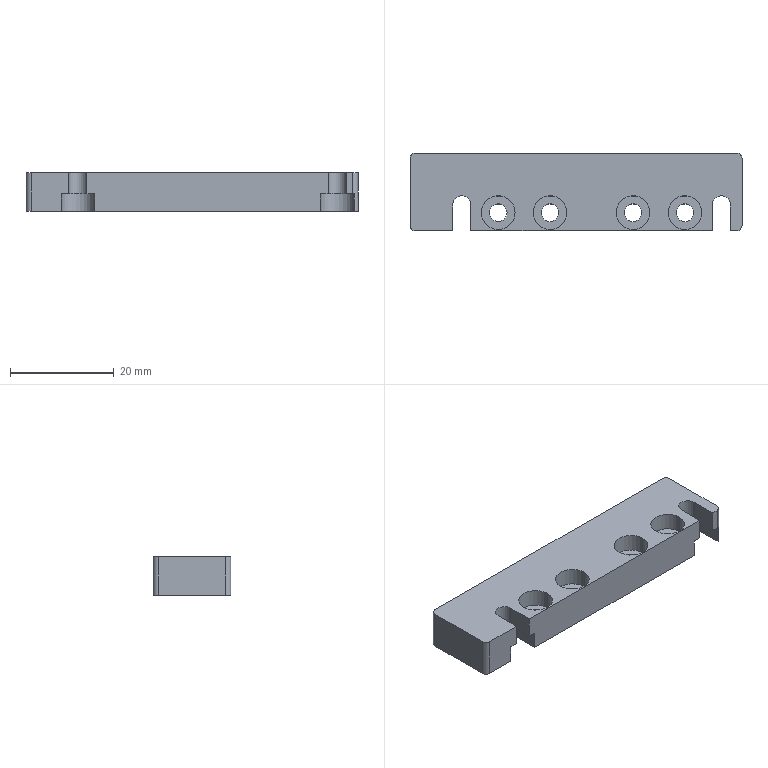Part | SolidWorks | features BaseBody 1 | 1 solid | 46 faces | box 64 x 15 x 7.5 mm | volume 6074 mm3 | cylinder 24 | plane 22 | commonest cylinder face diameters 6.5 x10 3.4 x8 2 x4 3.5 x2
STEP:
#1=CARTESIAN_POINT('',(-16.7,-4.,0.));
#2=VERTEX_POINT('',#1);
#3=CARTESIAN_POINT('',(-13.3,-4.,0.));
#4=VERTEX_POINT('',#3);
#5=CARTESIAN_POINT('',(-15.,-4.,0.));
#6=DIRECTION('',(0.,0.,1.));
#7=DIRECTION('',(1.,0.,0.));
#8=AXIS2_PLACEMENT_3D('',#5,#6,#7);
#9=CIRCLE('',#8,1.7);
#10=EDGE_CURVE('',#2,#4,#9,.T.);
#11=ORIENTED_EDGE('',*,*,#10,.F.);
#12=CARTESIAN_POINT('',(-16.7,-4.,4.1));
#13=VERTEX_POINT('',#12);
#14=CARTESIAN_POINT('',(-16.7,-4.,7.5));
#15=DIRECTION('',(0.,0.,1.));
#16=VECTOR('',#15,1000.);
#17=LINE('',#14,#16);
#18=EDGE_CURVE('',#2,#13,#17,.T.);
#19=ORIENTED_EDGE('',*,*,#18,.T.);
#20=CARTESIAN_POINT('',(-13.3,-4.,4.1));
#21=VERTEX_POINT('',#20);
#22=CARTESIAN_POINT('',(-15.,-4.,4.1));
#23=DIRECTION('',(0.,0.,-1.));
#24=DIRECTION('',(1.,0.,0.));
#25=AXIS2_PLACEMENT_3D('',#22,#23,#24);
#26=CIRCLE('',#25,1.7);
#27=EDGE_CURVE('',#21,#13,#26,.T.);
#28=ORIENTED_EDGE('',*,*,#27,.F.);
#29=CARTESIAN_POINT('',(-13.3,-4.,7.5));
#30=DIRECTION('',(0.,0.,1.));
#31=VECTOR('',#30,1000.);
#32=LINE('',#29,#31);
#33=EDGE_CURVE('',#4,#21,#32,.T.);
#34=ORIENTED_EDGE('',*,*,#33,.F.);
#35=EDGE_LOOP('',(#11,#19,#28,#34));
#36=FACE_OUTER_BOUND('',#35,.T.);
#37=CARTESIAN_POINT('',(-15.,-4.,7.5));
#38=DIRECTION('',(0.,0.,1.));
#39=DIRECTION('',(1.,0.,0.));
#40=AXIS2_PLACEMENT_3D('',#37,#38,#39);
#41=CYLINDRICAL_SURFACE('',#40,1.7);
#42=ADVANCED_FACE('',(#36),#41,.F.);
#43=CARTESIAN_POINT('',(9.3,-4.,0.));
#44=VERTEX_POINT('',#43);
#45=CARTESIAN_POINT('',(12.7,-4.,0.));
#46=VERTEX_POINT('',#45);
#47=CARTESIAN_POINT('',(11.,-4.,0.));
#48=DIRECTION('',(0.,0.,1.));
#49=DIRECTION('',(1.,0.,0.));
#50=AXIS2_PLACEMENT_3D('',#47,#48,#49);
#51=CIRCLE('',#50,1.7);
#52=EDGE_CURVE('',#44,#46,#51,.T.);
#53=ORIENTED_EDGE('',*,*,#52,.F.);
#54=CARTESIAN_POINT('',(9.3,-4.,4.1));
#55=VERTEX_POINT('',#54);
#56=CARTESIAN_POINT('',(9.3,-4.,7.5));
#57=DIRECTION('',(0.,0.,1.));
#58=VECTOR('',#57,1000.);
#59=LINE('',#56,#58);
#60=EDGE_CURVE('',#44,#55,#59,.T.);
#61=ORIENTED_EDGE('',*,*,#60,.T.);
#62=CARTESIAN_POINT('',(12.7,-4.,4.1));
#63=VERTEX_POINT('',#62);
#64=CARTESIAN_POINT('',(11.,-4.,4.1));
#65=DIRECTION('',(0.,0.,-1.));
#66=DIRECTION('',(1.,0.,0.));
#67=AXIS2_PLACEMENT_3D('',#64,#65,#66);
#68=CIRCLE('',#67,1.7);
#69=EDGE_CURVE('',#63,#55,#68,.T.);
#70=ORIENTED_EDGE('',*,*,#69,.F.);
#71=CARTESIAN_POINT('',(12.7,-4.,7.5));
#72=DIRECTION('',(0.,0.,1.));
#73=VECTOR('',#72,1000.);
#74=LINE('',#71,#73);
#75=EDGE_CURVE('',#46,#63,#74,.T.);
#76=ORIENTED_EDGE('',*,*,#75,.F.);
#77=EDGE_LOOP('',(#53,#61,#70,#76));
#78=FACE_OUTER_BOUND('',#77,.T.);
#79=CARTESIAN_POINT('',(11.,-4.,7.5));
#80=DIRECTION('',(0.,0.,1.));
#81=DIRECTION('',(1.,0.,0.));
#82=AXIS2_PLACEMENT_3D('',#79,#80,#81);
#83=CYLINDRICAL_SURFACE('',#82,1.7);
#84=ADVANCED_FACE('',(#78),#83,.F.);
#85=CARTESIAN_POINT('',(-6.7,-4.,0.));
#86=VERTEX_POINT('',#85);
#87=CARTESIAN_POINT('',(-3.3,-4.,0.));
#88=VERTEX_POINT('',#87);
#89=CARTESIAN_POINT('',(-5.,-4.,0.));
#90=DIRECTION('',(0.,0.,1.));
#91=DIRECTION('',(1.,0.,0.));
#92=AXIS2_PLACEMENT_3D('',#89,#90,#91);
#93=CIRCLE('',#92,1.7);
#94=EDGE_CURVE('',#86,#88,#93,.T.);
#95=ORIENTED_EDGE('',*,*,#94,.F.);
#96=CARTESIAN_POINT('',(-6.7,-4.,4.1));
#97=VERTEX_POINT('',#96);
#98=CARTESIAN_POINT('',(-6.7,-4.,7.5));
#99=DIRECTION('',(0.,0.,1.));
#100=VECTOR('',#99,1000.);
#101=LINE('',#98,#100);
#102=EDGE_CURVE('',#86,#97,#101,.T.);
#103=ORIENTED_EDGE('',*,*,#102,.T.);
#104=CARTESIAN_POINT('',(-3.3,-4.,4.1));
#105=VERTEX_POINT('',#104);
#106=CARTESIAN_POINT('',(-5.,-4.,4.1));
#107=DIRECTION('',(0.,0.,-1.));
#108=DIRECTION('',(1.,0.,0.));
#109=AXIS2_PLACEMENT_3D('',#106,#107,#108);
#110=CIRCLE('',#109,1.7);
#111=EDGE_CURVE('',#105,#97,#110,.T.);
#112=ORIENTED_EDGE('',*,*,#111,.F.);
#113=CARTESIAN_POINT('',(-3.3,-4.,7.5));
#114=DIRECTION('',(0.,0.,1.));
#115=VECTOR('',#114,1000.);
#116=LINE('',#113,#115);
#117=EDGE_CURVE('',#88,#105,#116,.T.);
#118=ORIENTED_EDGE('',*,*,#117,.F.);
#119=EDGE_LOOP('',(#95,#103,#112,#118));
#120=FACE_OUTER_BOUND('',#119,.T.);
#121=CARTESIAN_POINT('',(-5.,-4.,7.5));
#122=DIRECTION('',(0.,0.,1.));
#123=DIRECTION('',(1.,0.,0.));
#124=AXIS2_PLACEMENT_3D('',#121,#122,#123);
#125=CYLINDRICAL_SURFACE('',#124,1.7);
#126=ADVANCED_FACE('',(#120),#125,.F.);
#127=CARTESIAN_POINT('',(19.3,-4.,0.));
#128=VERTEX_POINT('',#127);
#129=CARTESIAN_POINT('',(22.7,-4.,0.));
#130=VERTEX_POINT('',#129);
#131=CARTESIAN_POINT('',(21.,-4.,0.));
#132=DIRECTION('',(0.,0.,1.));
#133=DIRECTION('',(1.,0.,0.));
#134=AXIS2_PLACEMENT_3D('',#131,#132,#133);
#135=CIRCLE('',#134,1.7);
#136=EDGE_CURVE('',#128,#130,#135,.T.);
#137=ORIENTED_EDGE('',*,*,#136,.F.);
#138=CARTESIAN_POINT('',(19.3,-4.,4.1));
#139=VERTEX_POINT('',#138);
#140=CARTESIAN_POINT('',(19.3,-4.,7.5));
#141=DIRECTION('',(0.,0.,1.));
#142=VECTOR('',#141,1000.);
#143=LINE('',#140,#142);
#144=EDGE_CURVE('',#128,#139,#143,.T.);
#145=ORIENTED_EDGE('',*,*,#144,.T.);
#146=CARTESIAN_POINT('',(22.7,-4.,4.1));
#147=VERTEX_POINT('',#146);
#148=CARTESIAN_POINT('',(21.,-4.,4.1));
#149=DIRECTION('',(0.,0.,-1.));
#150=DIRECTION('',(1.,0.,0.));
#151=AXIS2_PLACEMENT_3D('',#148,#149,#150);
#152=CIRCLE('',#151,1.7);
#153=EDGE_CURVE('',#147,#139,#152,.T.);
#154=ORIENTED_EDGE('',*,*,#153,.F.);
#155=CARTESIAN_POINT('',(22.7,-4.,7.5));
#156=DIRECTION('',(0.,0.,1.));
#157=VECTOR('',#156,1000.);
#158=LINE('',#155,#157);
#159=EDGE_CURVE('',#130,#147,#158,.T.);
#160=ORIENTED_EDGE('',*,*,#159,.F.);
#161=EDGE_LOOP('',(#137,#145,#154,#160));
#162=FACE_OUTER_BOUND('',#161,.T.);
#163=CARTESIAN_POINT('',(21.,-4.,7.5));
#164=DIRECTION('',(0.,0.,1.));
#165=DIRECTION('',(1.,0.,0.));
#166=AXIS2_PLACEMENT_3D('',#163,#164,#165);
#167=CYLINDRICAL_SURFACE('',#166,1.7);
#168=ADVANCED_FACE('',(#162),#167,.F.);
#169=CARTESIAN_POINT('',(-11.75,-4.,4.1));
#170=VERTEX_POINT('',#169);
#171=CARTESIAN_POINT('',(-18.25,-4.,4.1));
#172=VERTEX_POINT('',#171);
#173=CARTESIAN_POINT('',(-15.,-4.,4.1));
#174=DIRECTION('',(0.,0.,-1.));
#175=DIRECTION('',(1.,0.,0.));
#176=AXIS2_PLACEMENT_3D('',#173,#174,#175);
#177=CIRCLE('',#176,3.25);
#178=EDGE_CURVE('',#170,#172,#177,.T.);
#179=ORIENTED_EDGE('',*,*,#178,.T.);
#180=CARTESIAN_POINT('',(-18.25,-4.,7.5));
#181=VERTEX_POINT('',#180);
#182=CARTESIAN_POINT('',(-18.25,-4.,7.5));
#183=DIRECTION('',(0.,0.,1.));
#184=VECTOR('',#183,1000.);
#185=LINE('',#182,#184);
#186=EDGE_CURVE('',#172,#181,#185,.T.);
#187=ORIENTED_EDGE('',*,*,#186,.T.);
#188=CARTESIAN_POINT('',(-11.75,-4.,7.5));
#189=VERTEX_POINT('',#188);
#190=CARTESIAN_POINT('',(-15.,-4.,7.5));
#191=DIRECTION('',(0.,0.,1.));
#192=DIRECTION('',(1.,0.,0.));
#193=AXIS2_PLACEMENT_3D('',#190,#191,#192);
#194=CIRCLE('',#193,3.25);
#195=EDGE_CURVE('',#181,#189,#194,.T.);
#196=ORIENTED_EDGE('',*,*,#195,.T.);
#197=CARTESIAN_POINT('',(-11.75,-4.,7.5));
#198=DIRECTION('',(0.,0.,1.));
#199=VECTOR('',#198,1000.);
#200=LINE('',#197,#199);
#201=EDGE_CURVE('',#170,#189,#200,.T.);
#202=ORIENTED_EDGE('',*,*,#201,.F.);
#203=EDGE_LOOP('',(#179,#187,#196,#202));
#204=FACE_OUTER_BOUND('',#203,.T.);
#205=CARTESIAN_POINT('',(-15.,-4.,7.5));
#206=DIRECTION('',(0.,0.,1.));
#207=DIRECTION('',(1.,0.,0.));
#208=AXIS2_PLACEMENT_3D('',#205,#206,#207);
#209=CYLINDRICAL_SURFACE('',#208,3.25);
#210=ADVANCED_FACE('',(#204),#209,.F.);
#211=CARTESIAN_POINT('',(14.25,-4.,4.1));
#212=VERTEX_POINT('',#211);
#213=CARTESIAN_POINT('',(7.75,-4.,4.1));
#214=VERTEX_POINT('',#213);
#215=CARTESIAN_POINT('',(11.,-4.,4.1));
#216=DIRECTION('',(0.,0.,-1.));
#217=DIRECTION('',(1.,0.,0.));
#218=AXIS2_PLACEMENT_3D('',#215,#216,#217);
#219=CIRCLE('',#218,3.25);
#220=EDGE_CURVE('',#212,#214,#219,.T.);
#221=ORIENTED_EDGE('',*,*,#220,.T.);
#222=CARTESIAN_POINT('',(7.75,-4.,7.5));
#223=VERTEX_POINT('',#222);
#224=CARTESIAN_POINT('',(7.75,-4.,7.5));
#225=DIRECTION('',(0.,0.,1.));
#226=VECTOR('',#225,1000.);
#227=LINE('',#224,#226);
#228=EDGE_CURVE('',#214,#223,#227,.T.);
#229=ORIENTED_EDGE('',*,*,#228,.T.);
#230=CARTESIAN_POINT('',(14.25,-4.,7.5));
#231=VERTEX_POINT('',#230);
#232=CARTESIAN_POINT('',(11.,-4.,7.5));
#233=DIRECTION('',(0.,0.,1.));
#234=DIRECTION('',(1.,0.,0.));
#235=AXIS2_PLACEMENT_3D('',#232,#233,#234);
#236=CIRCLE('',#235,3.25);
#237=EDGE_CURVE('',#223,#231,#236,.T.);
#238=ORIENTED_EDGE('',*,*,#237,.T.);
#239=CARTESIAN_POINT('',(14.25,-4.,7.5));
#240=DIRECTION('',(0.,0.,1.));
#241=VECTOR('',#240,1000.);
#242=LINE('',#239,#241);
#243=EDGE_CURVE('',#212,#231,#242,.T.);
#244=ORIENTED_EDGE('',*,*,#243,.F.);
#245=EDGE_LOOP('',(#221,#229,#238,#244));
#246=FACE_OUTER_BOUND('',#245,.T.);
#247=CARTESIAN_POINT('',(11.,-4.,7.5));
#248=DIRECTION('',(0.,0.,1.));
#249=DIRECTION('',(1.,0.,0.));
#250=AXIS2_PLACEMENT_3D('',#247,#248,#249);
#251=CYLINDRICAL_SURFACE('',#250,3.25);
#252=ADVANCED_FACE('',(#246),#251,.F.);
#253=CARTESIAN_POINT('',(-1.75,-4.,4.1));
#254=VERTEX_POINT('',#253);
#255=CARTESIAN_POINT('',(-8.25,-4.,4.1));
#256=VERTEX_POINT('',#255);
#257=CARTESIAN_POINT('',(-5.,-4.,4.1));
#258=DIRECTION('',(0.,0.,-1.));
#259=DIRECTION('',(1.,0.,0.));
#260=AXIS2_PLACEMENT_3D('',#257,#258,#259);
#261=CIRCLE('',#260,3.25);
#262=EDGE_CURVE('',#254,#256,#261,.T.);
#263=ORIENTED_EDGE('',*,*,#262,.T.);
#264=CARTESIAN_POINT('',(-8.25,-4.,7.5));
#265=VERTEX_POINT('',#264);
#266=CARTESIAN_POINT('',(-8.25,-4.,7.5));
#267=DIRECTION('',(0.,0.,1.));
#268=VECTOR('',#267,1000.);
#269=LINE('',#266,#268);
#270=EDGE_CURVE('',#256,#265,#269,.T.);
#271=ORIENTED_EDGE('',*,*,#270,.T.);
#272=CARTESIAN_POINT('',(-1.75,-4.,7.5));
#273=VERTEX_POINT('',#272);
#274=CARTESIAN_POINT('',(-5.,-4.,7.5));
#275=DIRECTION('',(0.,0.,1.));
#276=DIRECTION('',(1.,0.,0.));
#277=AXIS2_PLACEMENT_3D('',#274,#275,#276);
#278=CIRCLE('',#277,3.25);
#279=EDGE_CURVE('',#265,#273,#278,.T.);
#280=ORIENTED_EDGE('',*,*,#279,.T.);
#281=CARTESIAN_POINT('',(-1.75,-4.,7.5));
#282=DIRECTION('',(0.,0.,1.));
#283=VECTOR('',#282,1000.);
#284=LINE('',#281,#283);
#285=EDGE_CURVE('',#254,#273,#284,.T.);
#286=ORIENTED_EDGE('',*,*,#285,.F.);
#287=EDGE_LOOP('',(#263,#271,#280,#286));
#288=FACE_OUTER_BOUND('',#287,.T.);
#289=CARTESIAN_POINT('',(-5.,-4.,7.5));
#290=DIRECTION('',(0.,0.,1.));
#291=DIRECTION('',(1.,0.,0.));
#292=AXIS2_PLACEMENT_3D('',#289,#290,#291);
#293=CYLINDRICAL_SURFACE('',#292,3.25);
#294=ADVANCED_FACE('',(#288),#293,.F.);
#295=CARTESIAN_POINT('',(24.25,-4.,4.1));
#296=VERTEX_POINT('',#295);
#297=CARTESIAN_POINT('',(17.75,-4.,4.1));
#298=VERTEX_POINT('',#297);
#299=CARTESIAN_POINT('',(21.,-4.,4.1));
#300=DIRECTION('',(0.,0.,-1.));
#301=DIRECTION('',(1.,0.,0.));
#302=AXIS2_PLACEMENT_3D('',#299,#300,#301);
#303=CIRCLE('',#302,3.25);
#304=EDGE_CURVE('',#296,#298,#303,.T.);
#305=ORIENTED_EDGE('',*,*,#304,.T.);
#306=CARTESIAN_POINT('',(17.75,-4.,7.5));
#307=VERTEX_POINT('',#306);
#308=CARTESIAN_POINT('',(17.75,-4.,7.5));
#309=DIRECTION('',(0.,0.,1.));
#310=VECTOR('',#309,1000.);
#311=LINE('',#308,#310);
#312=EDGE_CURVE('',#298,#307,#311,.T.);
#313=ORIENTED_EDGE('',*,*,#312,.T.);
#314=CARTESIAN_POINT('',(24.25,-4.,7.5));
#315=VERTEX_POINT('',#314);
#316=CARTESIAN_POINT('',(21.,-4.,7.5));
#317=DIRECTION('',(0.,0.,1.));
#318=DIRECTION('',(1.,0.,0.));
#319=AXIS2_PLACEMENT_3D('',#316,#317,#318);
#320=CIRCLE('',#319,3.25);
#321=EDGE_CURVE('',#307,#315,#320,.T.);
#322=ORIENTED_EDGE('',*,*,#321,.T.);
#323=CARTESIAN_POINT('',(24.25,-4.,7.5));
#324=DIRECTION('',(0.,0.,1.));
#325=VECTOR('',#324,1000.);
#326=LINE('',#323,#325);
#327=EDGE_CURVE('',#296,#315,#326,.T.);
#328=ORIENTED_EDGE('',*,*,#327,.F.);
#329=EDGE_LOOP('',(#305,#313,#322,#328));
#330=FACE_OUTER_BOUND('',#329,.T.);
#331=CARTESIAN_POINT('',(21.,-4.,7.5));
#332=DIRECTION('',(0.,0.,1.));
#333=DIRECTION('',(1.,0.,0.));
#334=AXIS2_PLACEMENT_3D('',#331,#332,#333);
#335=CYLINDRICAL_SURFACE('',#334,3.25);
#336=ADVANCED_FACE('',(#330),#335,.F.);
#337=CARTESIAN_POINT('',(-15.,-4.,0.));
#338=DIRECTION('',(0.,0.,1.));
#339=DIRECTION('',(1.,0.,0.));
#340=AXIS2_PLACEMENT_3D('',#337,#338,#339);
#341=CIRCLE('',#340,1.7);
#342=EDGE_CURVE('',#4,#2,#341,.T.);
#343=ORIENTED_EDGE('',*,*,#342,.T.);
#344=ORIENTED_EDGE('',*,*,#10,.T.);
#345=EDGE_LOOP('',(#343,#344));
#346=FACE_BOUND('',#345,.T.);
#347=CARTESIAN_POINT('',(11.,-4.,0.));
#348=DIRECTION('',(0.,0.,1.));
#349=DIRECTION('',(1.,0.,0.));
#350=AXIS2_PLACEMENT_3D('',#347,#348,#349);
#351=CIRCLE('',#350,1.7);
#352=EDGE_CURVE('',#46,#44,#351,.T.);
#353=ORIENTED_EDGE('',*,*,#352,.T.);
#354=ORIENTED_EDGE('',*,*,#52,.T.);
#355=EDGE_LOOP('',(#353,#354));
#356=FACE_BOUND('',#355,.T.);
#357=CARTESIAN_POINT('',(-5.,-4.,0.));
#358=DIRECTION('',(0.,0.,1.));
#359=DIRECTION('',(1.,0.,0.));
#360=AXIS2_PLACEMENT_3D('',#357,#358,#359);
#361=CIRCLE('',#360,1.7);
#362=EDGE_CURVE('',#88,#86,#361,.T.);
#363=ORIENTED_EDGE('',*,*,#362,.T.);
#364=ORIENTED_EDGE('',*,*,#94,.T.);
#365=EDGE_LOOP('',(#363,#364));
#366=FACE_BOUND('',#365,.T.);
#367=CARTESIAN_POINT('',(21.,-4.,0.));
#368=DIRECTION('',(0.,0.,1.));
#369=DIRECTION('',(1.,0.,0.));
#370=AXIS2_PLACEMENT_3D('',#367,#368,#369);
#371=CIRCLE('',#370,1.7);
#372=EDGE_CURVE('',#130,#128,#371,.T.);
#373=ORIENTED_EDGE('',*,*,#372,.T.);
#374=ORIENTED_EDGE('',*,*,#136,.T.);
#375=EDGE_LOOP('',(#373,#374));
#376=FACE_BOUND('',#375,.T.);
#377=CARTESIAN_POINT('',(31.25,-7.468,0.));
#378=VERTEX_POINT('',#377);
#379=CARTESIAN_POINT('',(31.25,-2.45,0.));
#380=VERTEX_POINT('',#379);
#381=CARTESIAN_POINT('',(31.25,0.,0.));
#382=DIRECTION('',(0.,1.,0.));
#383=VECTOR('',#382,1000.);
#384=LINE('',#381,#383);
#385=EDGE_CURVE('',#378,#380,#384,.T.);
#386=ORIENTED_EDGE('',*,*,#385,.T.);
#387=CARTESIAN_POINT('',(24.75,-2.45,0.));
#388=VERTEX_POINT('',#387);
#389=CARTESIAN_POINT('',(28.,-2.45,0.));
#390=DIRECTION('',(0.,0.,1.));
#391=DIRECTION('',(-1.,0.,0.));
#392=AXIS2_PLACEMENT_3D('',#389,#390,#391);
#393=CIRCLE('',#392,3.25);
#394=EDGE_CURVE('',#380,#388,#393,.T.);
#395=ORIENTED_EDGE('',*,*,#394,.T.);
#396=CARTESIAN_POINT('',(24.75,-7.5,0.));
#397=VERTEX_POINT('',#396);
#398=CARTESIAN_POINT('',(24.75,0.,0.));
#399=DIRECTION('',(0.,-1.,0.));
#400=VECTOR('',#399,1000.);
#401=LINE('',#398,#400);
#402=EDGE_CURVE('',#388,#397,#401,.T.);
#403=ORIENTED_EDGE('',*,*,#402,.T.);
#404=CARTESIAN_POINT('',(-18.75,-7.5,0.));
#405=VERTEX_POINT('',#404);
#406=CARTESIAN_POINT('',(0.,-7.5,0.));
#407=DIRECTION('',(-1.,0.,0.));
#408=VECTOR('',#407,1000.);
#409=LINE('',#406,#408);
#410=EDGE_CURVE('',#397,#405,#409,.T.);
#411=ORIENTED_EDGE('',*,*,#410,.T.);
#412=CARTESIAN_POINT('',(-18.75,-2.45,0.));
#413=VERTEX_POINT('',#412);
#414=CARTESIAN_POINT('',(-18.75,0.,0.));
#415=DIRECTION('',(0.,1.,0.));
#416=VECTOR('',#415,1000.);
#417=LINE('',#414,#416);
#418=EDGE_CURVE('',#405,#413,#417,.T.);
#419=ORIENTED_EDGE('',*,*,#418,.T.);
#420=CARTESIAN_POINT('',(-25.25,-2.45,0.));
#421=VERTEX_POINT('',#420);
#422=CARTESIAN_POINT('',(-22.,-2.45,0.));
#423=DIRECTION('',(0.,0.,1.));
#424=DIRECTION('',(-1.,0.,0.));
#425=AXIS2_PLACEMENT_3D('',#422,#423,#424);
#426=CIRCLE('',#425,3.25);
#427=EDGE_CURVE('',#413,#421,#426,.T.);
#428=ORIENTED_EDGE('',*,*,#427,.T.);
#429=CARTESIAN_POINT('',(-25.25,-7.5,0.));
#430=VERTEX_POINT('',#429);
#431=CARTESIAN_POINT('',(-25.25,0.,0.));
#432=DIRECTION('',(0.,-1.,0.));
#433=VECTOR('',#432,1000.);
#434=LINE('',#431,#433);
#435=EDGE_CURVE('',#421,#430,#434,.T.);
#436=ORIENTED_EDGE('',*,*,#435,.T.);
#437=CARTESIAN_POINT('',(-31.,-7.5,0.));
#438=VERTEX_POINT('',#437);
#439=CARTESIAN_POINT('',(0.,-7.5,0.));
#440=DIRECTION('',(-1.,0.,0.));
#441=VECTOR('',#440,1000.);
#442=LINE('',#439,#441);
#443=EDGE_CURVE('',#430,#438,#442,.T.);
#444=ORIENTED_EDGE('',*,*,#443,.T.);
#445=CARTESIAN_POINT('',(-32.,-6.5,0.));
#446=VERTEX_POINT('',#445);
#447=CARTESIAN_POINT('',(-31.,-6.5,0.));
#448=DIRECTION('',(0.,0.,1.));
#449=DIRECTION('',(-1.,0.,0.));
#450=AXIS2_PLACEMENT_3D('',#447,#448,#449);
#451=CIRCLE('',#450,1.);
#452=EDGE_CURVE('',#446,#438,#451,.T.);
#453=ORIENTED_EDGE('',*,*,#452,.F.);
#454=CARTESIAN_POINT('',(-32.,6.5,0.));
#455=VERTEX_POINT('',#454);
#456=CARTESIAN_POINT('',(-32.,0.,0.));
#457=DIRECTION('',(0.,1.,0.));
#458=VECTOR('',#457,1000.);
#459=LINE('',#456,#458);
#460=EDGE_CURVE('',#446,#455,#459,.T.);
#461=ORIENTED_EDGE('',*,*,#460,.T.);
#462=CARTESIAN_POINT('',(-31.,7.5,0.));
#463=VERTEX_POINT('',#462);
#464=CARTESIAN_POINT('',(-31.,6.5,0.));
#465=DIRECTION('',(0.,0.,1.));
#466=DIRECTION('',(-1.,0.,0.));
#467=AXIS2_PLACEMENT_3D('',#464,#465,#466);
#468=CIRCLE('',#467,1.);
#469=EDGE_CURVE('',#463,#455,#468,.T.);
#470=ORIENTED_EDGE('',*,*,#469,.F.);
#471=CARTESIAN_POINT('',(31.,7.5,0.));
#472=VERTEX_POINT('',#471);
#473=CARTESIAN_POINT('',(0.,7.5,0.));
#474=DIRECTION('',(1.,0.,0.));
#475=VECTOR('',#474,1000.);
#476=LINE('',#473,#475);
#477=EDGE_CURVE('',#463,#472,#476,.T.);
#478=ORIENTED_EDGE('',*,*,#477,.T.);
#479=CARTESIAN_POINT('',(32.,6.5,0.));
#480=VERTEX_POINT('',#479);
#481=CARTESIAN_POINT('',(31.,6.5,0.));
#482=DIRECTION('',(0.,0.,1.));
#483=DIRECTION('',(-1.,0.,0.));
#484=AXIS2_PLACEMENT_3D('',#481,#482,#483);
#485=CIRCLE('',#484,1.);
#486=EDGE_CURVE('',#480,#472,#485,.T.);
#487=ORIENTED_EDGE('',*,*,#486,.F.);
#488=CARTESIAN_POINT('',(32.,-6.5,0.));
#489=VERTEX_POINT('',#488);
#490=CARTESIAN_POINT('',(32.,0.,0.));
#491=DIRECTION('',(0.,-1.,0.));
#492=VECTOR('',#491,1000.);
#493=LINE('',#490,#492);
#494=EDGE_CURVE('',#480,#489,#493,.T.);
#495=ORIENTED_EDGE('',*,*,#494,.T.);
#496=CARTESIAN_POINT('',(31.,-6.5,0.));
#497=DIRECTION('',(0.,0.,1.));
#498=DIRECTION('',(-1.,0.,0.));
#499=AXIS2_PLACEMENT_3D('',#496,#497,#498);
#500=CIRCLE('',#499,1.);
#501=EDGE_CURVE('',#378,#489,#500,.T.);
#502=ORIENTED_EDGE('',*,*,#501,.F.);
#503=EDGE_LOOP('',(#386,#395,#403,#411,#419,#428,#436,#444,#453,#461,#470,#478,#487,#495,#502));
#504=FACE_OUTER_BOUND('',#503,.T.);
#505=CARTESIAN_POINT('',(0.,0.,0.));
#506=DIRECTION('',(0.,0.,-1.));
#507=DIRECTION('',(-1.,0.,0.));
#508=AXIS2_PLACEMENT_3D('',#505,#506,#507);
#509=PLANE('',#508);
#510=ADVANCED_FACE('',(#346,#356,#366,#376,#504),#509,.T.);
#511=ORIENTED_EDGE('',*,*,#18,.F.);
#512=ORIENTED_EDGE('',*,*,#342,.F.);
#513=ORIENTED_EDGE('',*,*,#33,.T.);
#514=CARTESIAN_POINT('',(-15.,-4.,4.1));
#515=DIRECTION('',(0.,0.,-1.));
#516=DIRECTION('',(1.,0.,0.));
#517=AXIS2_PLACEMENT_3D('',#514,#515,#516);
#518=CIRCLE('',#517,1.7);
#519=EDGE_CURVE('',#13,#21,#518,.T.);
#520=ORIENTED_EDGE('',*,*,#519,.F.);
#521=EDGE_LOOP('',(#511,#512,#513,#520));
#522=FACE_OUTER_BOUND('',#521,.T.);
#523=CARTESIAN_POINT('',(-15.,-4.,7.5));
#524=DIRECTION('',(0.,0.,1.));
#525=DIRECTION('',(1.,0.,0.));
#526=AXIS2_PLACEMENT_3D('',#523,#524,#525);
#527=CYLINDRICAL_SURFACE('',#526,1.7);
#528=ADVANCED_FACE('',(#522),#527,.F.);
#529=ORIENTED_EDGE('',*,*,#60,.F.);
#530=ORIENTED_EDGE('',*,*,#352,.F.);
#531=ORIENTED_EDGE('',*,*,#75,.T.);
#532=CARTESIAN_POINT('',(11.,-4.,4.1));
#533=DIRECTION('',(0.,0.,-1.));
#534=DIRECTION('',(1.,0.,0.));
#535=AXIS2_PLACEMENT_3D('',#532,#533,#534);
#536=CIRCLE('',#535,1.7);
#537=EDGE_CURVE('',#55,#63,#536,.T.);
#538=ORIENTED_EDGE('',*,*,#537,.F.);
#539=EDGE_LOOP('',(#529,#530,#531,#538));
#540=FACE_OUTER_BOUND('',#539,.T.);
#541=CARTESIAN_POINT('',(11.,-4.,7.5));
#542=DIRECTION('',(0.,0.,1.));
#543=DIRECTION('',(1.,0.,0.));
#544=AXIS2_PLACEMENT_3D('',#541,#542,#543);
#545=CYLINDRICAL_SURFACE('',#544,1.7);
#546=ADVANCED_FACE('',(#540),#545,.F.);
#547=ORIENTED_EDGE('',*,*,#102,.F.);
#548=ORIENTED_EDGE('',*,*,#362,.F.);
#549=ORIENTED_EDGE('',*,*,#117,.T.);
#550=CARTESIAN_POINT('',(-5.,-4.,4.1));
#551=DIRECTION('',(0.,0.,-1.));
#552=DIRECTION('',(1.,0.,0.));
#553=AXIS2_PLACEMENT_3D('',#550,#551,#552);
#554=CIRCLE('',#553,1.7);
#555=EDGE_CURVE('',#97,#105,#554,.T.);
#556=ORIENTED_EDGE('',*,*,#555,.F.);
#557=EDGE_LOOP('',(#547,#548,#549,#556));
#558=FACE_OUTER_BOUND('',#557,.T.);
#559=CARTESIAN_POINT('',(-5.,-4.,7.5));
#560=DIRECTION('',(0.,0.,1.));
#561=DIRECTION('',(1.,0.,0.));
#562=AXIS2_PLACEMENT_3D('',#559,#560,#561);
#563=CYLINDRICAL_SURFACE('',#562,1.7);
#564=ADVANCED_FACE('',(#558),#563,.F.);
#565=ORIENTED_EDGE('',*,*,#144,.F.);
#566=ORIENTED_EDGE('',*,*,#372,.F.);
#567=ORIENTED_EDGE('',*,*,#159,.T.);
#568=CARTESIAN_POINT('',(21.,-4.,4.1));
#569=DIRECTION('',(0.,0.,-1.));
#570=DIRECTION('',(1.,0.,0.));
#571=AXIS2_PLACEMENT_3D('',#568,#569,#570);
#572=CIRCLE('',#571,1.7);
#573=EDGE_CURVE('',#139,#147,#572,.T.);
#574=ORIENTED_EDGE('',*,*,#573,.F.);
#575=EDGE_LOOP('',(#565,#566,#567,#574));
#576=FACE_OUTER_BOUND('',#575,.T.);
#577=CARTESIAN_POINT('',(21.,-4.,7.5));
#578=DIRECTION('',(0.,0.,1.));
#579=DIRECTION('',(1.,0.,0.));
#580=AXIS2_PLACEMENT_3D('',#577,#578,#579);
#581=CYLINDRICAL_SURFACE('',#580,1.7);
#582=ADVANCED_FACE('',(#576),#581,.F.);
#583=CARTESIAN_POINT('',(31.25,-2.45,3.4));
#584=VERTEX_POINT('',#583);
#585=CARTESIAN_POINT('',(31.25,-2.45,0.));
#586=DIRECTION('',(0.,0.,-1.));
#587=VECTOR('',#586,1000.);
#588=LINE('',#585,#587);
#589=EDGE_CURVE('',#584,#380,#588,.T.);
#590=ORIENTED_EDGE('',*,*,#589,.F.);
#591=CARTESIAN_POINT('',(24.75,-2.45,3.4));
#592=VERTEX_POINT('',#591);
#593=CARTESIAN_POINT('',(28.,-2.45,3.4));
#594=DIRECTION('',(0.,0.,-1.));
#595=DIRECTION('',(-1.,0.,0.));
#596=AXIS2_PLACEMENT_3D('',#593,#594,#595);
#597=CIRCLE('',#596,3.25);
#598=EDGE_CURVE('',#592,#584,#597,.T.);
#599=ORIENTED_EDGE('',*,*,#598,.F.);
#600=CARTESIAN_POINT('',(24.75,-2.45,0.));
#601=DIRECTION('',(0.,0.,1.));
#602=VECTOR('',#601,1000.);
#603=LINE('',#600,#602);
#604=EDGE_CURVE('',#388,#592,#603,.T.);
#605=ORIENTED_EDGE('',*,*,#604,.F.);
#606=ORIENTED_EDGE('',*,*,#394,.F.);
#607=EDGE_LOOP('',(#590,#599,#605,#606));
#608=FACE_OUTER_BOUND('',#607,.T.);
#609=CARTESIAN_POINT('',(28.,-2.45,0.));
#610=DIRECTION('',(0.,0.,-1.));
#611=DIRECTION('',(-1.,0.,0.));
#612=AXIS2_PLACEMENT_3D('',#609,#610,#611);
#613=CYLINDRICAL_SURFACE('',#612,3.25);
#614=ADVANCED_FACE('',(#608),#613,.F.);
#615=ORIENTED_EDGE('',*,*,#385,.F.);
#616=CARTESIAN_POINT('',(31.25,-7.468,3.4));
#617=VERTEX_POINT('',#616);
#618=CARTESIAN_POINT('',(31.25,-7.468,3.4));
#619=DIRECTION('',(0.,0.,1.));
#620=VECTOR('',#619,1000.);
#621=LINE('',#618,#620);
#622=EDGE_CURVE('',#378,#617,#621,.T.);
#623=ORIENTED_EDGE('',*,*,#622,.T.);
#624=CARTESIAN_POINT('',(31.25,-9.05,3.4));
#625=DIRECTION('',(0.,1.,0.));
#626=VECTOR('',#625,1000.);
#627=LINE('',#624,#626);
#628=EDGE_CURVE('',#617,#584,#627,.T.);
#629=ORIENTED_EDGE('',*,*,#628,.T.);
#630=ORIENTED_EDGE('',*,*,#589,.T.);
#631=EDGE_LOOP('',(#615,#623,#629,#630));
#632=FACE_OUTER_BOUND('',#631,.T.);
#633=CARTESIAN_POINT('',(31.25,-9.05,3.4));
#634=DIRECTION('',(-1.,0.,0.));
#635=DIRECTION('',(0.,0.,1.));
#636=AXIS2_PLACEMENT_3D('',#633,#634,#635);
#637=PLANE('',#636);
#638=ADVANCED_FACE('',(#632),#637,.T.);
#639=CARTESIAN_POINT('',(32.,6.5,7.5));
#640=VERTEX_POINT('',#639);
#641=CARTESIAN_POINT('',(32.,6.5,7.5));
#642=DIRECTION('',(0.,0.,-1.));
#643=VECTOR('',#642,1000.);
#644=LINE('',#641,#643);
#645=EDGE_CURVE('',#640,#480,#644,.T.);
#646=ORIENTED_EDGE('',*,*,#645,.F.);
#647=CARTESIAN_POINT('',(32.,-6.5,7.5));
#648=VERTEX_POINT('',#647);
#649=CARTESIAN_POINT('',(32.,-7.5,7.5));
#650=DIRECTION('',(0.,1.,0.));
#651=VECTOR('',#650,1000.);
#652=LINE('',#649,#651);
#653=EDGE_CURVE('',#648,#640,#652,.T.);
#654=ORIENTED_EDGE('',*,*,#653,.F.);
#655=CARTESIAN_POINT('',(32.,-6.5,7.5));
#656=DIRECTION('',(0.,0.,1.));
#657=VECTOR('',#656,1000.);
#658=LINE('',#655,#657);
#659=EDGE_CURVE('',#489,#648,#658,.T.);
#660=ORIENTED_EDGE('',*,*,#659,.F.);
#661=ORIENTED_EDGE('',*,*,#494,.F.);
#662=EDGE_LOOP('',(#646,#654,#660,#661));
#663=FACE_OUTER_BOUND('',#662,.T.);
#664=CARTESIAN_POINT('',(32.,-7.5,7.5));
#665=DIRECTION('',(-1.,0.,0.));
#666=DIRECTION('',(0.,0.,1.));
#667=AXIS2_PLACEMENT_3D('',#664,#665,#666);
#668=PLANE('',#667);
#669=ADVANCED_FACE('',(#663),#668,.F.);
#670=CARTESIAN_POINT('',(31.,7.5,7.5));
#671=VERTEX_POINT('',#670);
#672=CARTESIAN_POINT('',(31.,7.5,7.5));
#673=DIRECTION('',(0.,0.,1.));
#674=VECTOR('',#673,1000.);
#675=LINE('',#672,#674);
#676=EDGE_CURVE('',#472,#671,#675,.T.);
#677=ORIENTED_EDGE('',*,*,#676,.F.);
#678=ORIENTED_EDGE('',*,*,#477,.F.);
#679=CARTESIAN_POINT('',(-31.,7.5,7.5));
#680=VERTEX_POINT('',#679);
#681=CARTESIAN_POINT('',(-31.,7.5,7.5));
#682=DIRECTION('',(0.,0.,-1.));
#683=VECTOR('',#682,1000.);
#684=LINE('',#681,#683);
#685=EDGE_CURVE('',#680,#463,#684,.T.);
#686=ORIENTED_EDGE('',*,*,#685,.F.);
#687=CARTESIAN_POINT('',(-32.,7.5,7.5));
#688=DIRECTION('',(-1.,0.,0.));
#689=VECTOR('',#688,1000.);
#690=LINE('',#687,#689);
#691=EDGE_CURVE('',#671,#680,#690,.T.);
#692=ORIENTED_EDGE('',*,*,#691,.F.);
#693=EDGE_LOOP('',(#677,#678,#686,#692));
#694=FACE_OUTER_BOUND('',#693,.T.);
#695=CARTESIAN_POINT('',(-32.,7.5,7.5));
#696=DIRECTION('',(0.,-1.,0.));
#697=DIRECTION('',(0.,0.,-1.));
#698=AXIS2_PLACEMENT_3D('',#695,#696,#697);
#699=PLANE('',#698);
#700=ADVANCED_FACE('',(#694),#699,.F.);
#701=CARTESIAN_POINT('',(-32.,-6.5,7.5));
#702=VERTEX_POINT('',#701);
#703=CARTESIAN_POINT('',(-32.,-6.5,7.5));
#704=DIRECTION('',(0.,0.,-1.));
#705=VECTOR('',#704,1000.);
#706=LINE('',#703,#705);
#707=EDGE_CURVE('',#702,#446,#706,.T.);
#708=ORIENTED_EDGE('',*,*,#707,.F.);
#709=CARTESIAN_POINT('',(-32.,6.5,7.5));
#710=VERTEX_POINT('',#709);
#711=CARTESIAN_POINT('',(-32.,-7.5,7.5));
#712=DIRECTION('',(0.,-1.,0.));
#713=VECTOR('',#712,1000.);
#714=LINE('',#711,#713);
#715=EDGE_CURVE('',#710,#702,#714,.T.);
#716=ORIENTED_EDGE('',*,*,#715,.F.);
#717=CARTESIAN_POINT('',(-32.,6.5,7.5));
#718=DIRECTION('',(0.,0.,1.));
#719=VECTOR('',#718,1000.);
#720=LINE('',#717,#719);
#721=EDGE_CURVE('',#455,#710,#720,.T.);
#722=ORIENTED_EDGE('',*,*,#721,.F.);
#723=ORIENTED_EDGE('',*,*,#460,.F.);
#724=EDGE_LOOP('',(#708,#716,#722,#723));
#725=FACE_OUTER_BOUND('',#724,.T.);
#726=CARTESIAN_POINT('',(-32.,-7.5,7.5));
#727=DIRECTION('',(1.,0.,0.));
#728=DIRECTION('',(0.,0.,-1.));
#729=AXIS2_PLACEMENT_3D('',#726,#727,#728);
#730=PLANE('',#729);
#731=ADVANCED_FACE('',(#725),#730,.F.);
#732=CARTESIAN_POINT('',(-25.25,-7.5,3.4));
#733=VERTEX_POINT('',#732);
#734=CARTESIAN_POINT('',(-23.75,-7.5,3.4));
#735=VERTEX_POINT('',#734);
#736=CARTESIAN_POINT('',(-20.3,-7.5,3.4));
#737=DIRECTION('',(1.,0.,0.));
#738=VECTOR('',#737,1000.);
#739=LINE('',#736,#738);
#740=EDGE_CURVE('',#733,#735,#739,.T.);
#741=ORIENTED_EDGE('',*,*,#740,.T.);
#742=CARTESIAN_POINT('',(-23.75,-7.5,7.5));
#743=VERTEX_POINT('',#742);
#744=CARTESIAN_POINT('',(-23.75,-7.5,7.5));
#745=DIRECTION('',(0.,0.,-1.));
#746=VECTOR('',#745,1000.);
#747=LINE('',#744,#746);
#748=EDGE_CURVE('',#743,#735,#747,.T.);
#749=ORIENTED_EDGE('',*,*,#748,.F.);
#750=CARTESIAN_POINT('',(-31.,-7.5,7.5));
#751=VERTEX_POINT('',#750);
#752=CARTESIAN_POINT('',(-32.,-7.5,7.5));
#753=DIRECTION('',(1.,0.,0.));
#754=VECTOR('',#753,1000.);
#755=LINE('',#752,#754);
#756=EDGE_CURVE('',#751,#743,#755,.T.);
#757=ORIENTED_EDGE('',*,*,#756,.F.);
#758=CARTESIAN_POINT('',(-31.,-7.5,7.5));
#759=DIRECTION('',(0.,0.,1.));
#760=VECTOR('',#759,1000.);
#761=LINE('',#758,#760);
#762=EDGE_CURVE('',#438,#751,#761,.T.);
#763=ORIENTED_EDGE('',*,*,#762,.F.);
#764=ORIENTED_EDGE('',*,*,#443,.F.);
#765=CARTESIAN_POINT('',(-25.25,-7.5,7.5));
#766=DIRECTION('',(0.,0.,-1.));
#767=VECTOR('',#766,1000.);
#768=LINE('',#765,#767);
#769=EDGE_CURVE('',#733,#430,#768,.T.);
#770=ORIENTED_EDGE('',*,*,#769,.F.);
#771=EDGE_LOOP('',(#741,#749,#757,#763,#764,#770));
#772=FACE_OUTER_BOUND('',#771,.T.);
#773=CARTESIAN_POINT('',(-32.,-7.5,7.5));
#774=DIRECTION('',(0.,1.,0.));
#775=DIRECTION('',(0.,0.,1.));
#776=AXIS2_PLACEMENT_3D('',#773,#774,#775);
#777=PLANE('',#776);
#778=ADVANCED_FACE('',(#772),#777,.F.);
#779=CARTESIAN_POINT('',(-25.25,-2.45,3.4));
#780=VERTEX_POINT('',#779);
#781=CARTESIAN_POINT('',(-25.25,-2.45,0.));
#782=DIRECTION('',(0.,0.,-1.));
#783=VECTOR('',#782,1000.);
#784=LINE('',#781,#783);
#785=EDGE_CURVE('',#780,#421,#784,.T.);
#786=ORIENTED_EDGE('',*,*,#785,.F.);
#787=CARTESIAN_POINT('',(-25.25,-9.05,3.4));
#788=DIRECTION('',(0.,1.,0.));
#789=VECTOR('',#788,1000.);
#790=LINE('',#787,#789);
#791=EDGE_CURVE('',#733,#780,#790,.T.);
#792=ORIENTED_EDGE('',*,*,#791,.F.);
#793=ORIENTED_EDGE('',*,*,#769,.T.);
#794=ORIENTED_EDGE('',*,*,#435,.F.);
#795=EDGE_LOOP('',(#786,#792,#793,#794));
#796=FACE_OUTER_BOUND('',#795,.T.);
#797=CARTESIAN_POINT('',(-25.25,-9.05,0.));
#798=DIRECTION('',(-1.,0.,0.));
#799=DIRECTION('',(0.,0.,1.));
#800=AXIS2_PLACEMENT_3D('',#797,#798,#799);
#801=PLANE('',#800);
#802=ADVANCED_FACE('',(#796),#801,.F.);
#803=CARTESIAN_POINT('',(-18.75,-2.45,3.4));
#804=VERTEX_POINT('',#803);
#805=CARTESIAN_POINT('',(-18.75,-2.45,0.));
#806=DIRECTION('',(0.,0.,-1.));
#807=VECTOR('',#806,1000.);
#808=LINE('',#805,#807);
#809=EDGE_CURVE('',#804,#413,#808,.T.);
#810=ORIENTED_EDGE('',*,*,#809,.F.);
#811=CARTESIAN_POINT('',(-22.,-2.45,3.4));
#812=DIRECTION('',(0.,0.,-1.));
#813=DIRECTION('',(-1.,0.,0.));
#814=AXIS2_PLACEMENT_3D('',#811,#812,#813);
#815=CIRCLE('',#814,3.25);
#816=EDGE_CURVE('',#780,#804,#815,.T.);
#817=ORIENTED_EDGE('',*,*,#816,.F.);
#818=ORIENTED_EDGE('',*,*,#785,.T.);
#819=ORIENTED_EDGE('',*,*,#427,.F.);
#820=EDGE_LOOP('',(#810,#817,#818,#819));
#821=FACE_OUTER_BOUND('',#820,.T.);
#822=CARTESIAN_POINT('',(-22.,-2.45,0.));
#823=DIRECTION('',(0.,0.,-1.));
#824=DIRECTION('',(-1.,0.,0.));
#825=AXIS2_PLACEMENT_3D('',#822,#823,#824);
#826=CYLINDRICAL_SURFACE('',#825,3.25);
#827=ADVANCED_FACE('',(#821),#826,.F.);
#828=ORIENTED_EDGE('',*,*,#809,.T.);
#829=ORIENTED_EDGE('',*,*,#418,.F.);
#830=CARTESIAN_POINT('',(-18.75,-7.5,3.4));
#831=VERTEX_POINT('',#830);
#832=CARTESIAN_POINT('',(-18.75,-7.5,3.4));
#833=DIRECTION('',(0.,0.,1.));
#834=VECTOR('',#833,1000.);
#835=LINE('',#832,#834);
#836=EDGE_CURVE('',#405,#831,#835,.T.);
#837=ORIENTED_EDGE('',*,*,#836,.T.);
#838=CARTESIAN_POINT('',(-18.75,-9.05,3.4));
#839=DIRECTION('',(0.,1.,0.));
#840=VECTOR('',#839,1000.);
#841=LINE('',#838,#840);
#842=EDGE_CURVE('',#831,#804,#841,.T.);
#843=ORIENTED_EDGE('',*,*,#842,.T.);
#844=EDGE_LOOP('',(#828,#829,#837,#843));
#845=FACE_OUTER_BOUND('',#844,.T.);
#846=CARTESIAN_POINT('',(-18.75,-9.05,3.4));
#847=DIRECTION('',(-1.,0.,0.));
#848=DIRECTION('',(0.,0.,1.));
#849=AXIS2_PLACEMENT_3D('',#846,#847,#848);
#850=PLANE('',#849);
#851=ADVANCED_FACE('',(#845),#850,.T.);
#852=CARTESIAN_POINT('',(24.75,-7.5,3.4));
#853=VERTEX_POINT('',#852);
#854=CARTESIAN_POINT('',(24.75,-7.5,7.5));
#855=DIRECTION('',(0.,0.,-1.));
#856=VECTOR('',#855,1000.);
#857=LINE('',#854,#856);
#858=EDGE_CURVE('',#853,#397,#857,.T.);
#859=ORIENTED_EDGE('',*,*,#858,.F.);
#860=CARTESIAN_POINT('',(26.25,-7.5,3.4));
#861=VERTEX_POINT('',#860);
#862=CARTESIAN_POINT('',(-32.,-7.5,3.4));
#863=DIRECTION('',(-1.,0.,0.));
#864=VECTOR('',#863,1000.);
#865=LINE('',#862,#864);
#866=EDGE_CURVE('',#861,#853,#865,.T.);
#867=ORIENTED_EDGE('',*,*,#866,.F.);
#868=CARTESIAN_POINT('',(26.25,-7.5,7.5));
#869=VERTEX_POINT('',#868);
#870=CARTESIAN_POINT('',(26.25,-7.5,7.5));
#871=DIRECTION('',(0.,0.,-1.));
#872=VECTOR('',#871,1000.);
#873=LINE('',#870,#872);
#874=EDGE_CURVE('',#869,#861,#873,.T.);
#875=ORIENTED_EDGE('',*,*,#874,.F.);
#876=CARTESIAN_POINT('',(-20.25,-7.5,7.5));
#877=VERTEX_POINT('',#876);
#878=CARTESIAN_POINT('',(-32.,-7.5,7.5));
#879=DIRECTION('',(1.,0.,0.));
#880=VECTOR('',#879,1000.);
#881=LINE('',#878,#880);
#882=EDGE_CURVE('',#877,#869,#881,.T.);
#883=ORIENTED_EDGE('',*,*,#882,.F.);
#884=CARTESIAN_POINT('',(-20.25,-7.5,3.4));
#885=VERTEX_POINT('',#884);
#886=CARTESIAN_POINT('',(-20.25,-7.5,7.5));
#887=DIRECTION('',(0.,0.,1.));
#888=VECTOR('',#887,1000.);
#889=LINE('',#886,#888);
#890=EDGE_CURVE('',#885,#877,#889,.T.);
#891=ORIENTED_EDGE('',*,*,#890,.F.);
#892=CARTESIAN_POINT('',(-32.,-7.5,3.4));
#893=DIRECTION('',(-1.,0.,0.));
#894=VECTOR('',#893,1000.);
#895=LINE('',#892,#894);
#896=EDGE_CURVE('',#831,#885,#895,.T.);
#897=ORIENTED_EDGE('',*,*,#896,.F.);
#898=ORIENTED_EDGE('',*,*,#836,.F.);
#899=ORIENTED_EDGE('',*,*,#410,.F.);
#900=EDGE_LOOP('',(#859,#867,#875,#883,#891,#897,#898,#899));
#901=FACE_OUTER_BOUND('',#900,.T.);
#902=CARTESIAN_POINT('',(-32.,-7.5,7.5));
#903=DIRECTION('',(0.,1.,0.));
#904=DIRECTION('',(0.,0.,1.));
#905=AXIS2_PLACEMENT_3D('',#902,#903,#904);
#906=PLANE('',#905);
#907=ADVANCED_FACE('',(#901),#906,.F.);
#908=ORIENTED_EDGE('',*,*,#604,.T.);
#909=CARTESIAN_POINT('',(24.75,-9.05,3.4));
#910=DIRECTION('',(0.,1.,0.));
#911=VECTOR('',#910,1000.);
#912=LINE('',#909,#911);
#913=EDGE_CURVE('',#853,#592,#912,.T.);
#914=ORIENTED_EDGE('',*,*,#913,.F.);
#915=ORIENTED_EDGE('',*,*,#858,.T.);
#916=ORIENTED_EDGE('',*,*,#402,.F.);
#917=EDGE_LOOP('',(#908,#914,#915,#916));
#918=FACE_OUTER_BOUND('',#917,.T.);
#919=CARTESIAN_POINT('',(24.75,-9.05,0.));
#920=DIRECTION('',(-1.,0.,0.));
#921=DIRECTION('',(0.,0.,1.));
#922=AXIS2_PLACEMENT_3D('',#919,#920,#921);
#923=PLANE('',#922);
#924=ADVANCED_FACE('',(#918),#923,.F.);
#925=ORIENTED_EDGE('',*,*,#178,.F.);
#926=CARTESIAN_POINT('',(-15.,-4.,4.1));
#927=DIRECTION('',(0.,0.,-1.));
#928=DIRECTION('',(1.,0.,0.));
#929=AXIS2_PLACEMENT_3D('',#926,#927,#928);
#930=CIRCLE('',#929,3.25);
#931=EDGE_CURVE('',#172,#170,#930,.T.);
#932=ORIENTED_EDGE('',*,*,#931,.F.);
#933=EDGE_LOOP('',(#925,#932));
#934=FACE_OUTER_BOUND('',#933,.T.);
#935=ORIENTED_EDGE('',*,*,#27,.T.);
#936=ORIENTED_EDGE('',*,*,#519,.T.);
#937=EDGE_LOOP('',(#935,#936));
#938=FACE_BOUND('',#937,.T.);
#939=CARTESIAN_POINT('',(-13.3,-4.,4.1));
#940=DIRECTION('',(0.,0.,-1.));
#941=DIRECTION('',(-1.,0.,0.));
#942=AXIS2_PLACEMENT_3D('',#939,#940,#941);
#943=PLANE('',#942);
#944=ADVANCED_FACE('',(#934,#938),#943,.F.);
#945=ORIENTED_EDGE('',*,*,#220,.F.);
#946=CARTESIAN_POINT('',(11.,-4.,4.1));
#947=DIRECTION('',(0.,0.,-1.));
#948=DIRECTION('',(1.,0.,0.));
#949=AXIS2_PLACEMENT_3D('',#946,#947,#948);
#950=CIRCLE('',#949,3.25);
#951=EDGE_CURVE('',#214,#212,#950,.T.);
#952=ORIENTED_EDGE('',*,*,#951,.F.);
#953=EDGE_LOOP('',(#945,#952));
#954=FACE_OUTER_BOUND('',#953,.T.);
#955=ORIENTED_EDGE('',*,*,#69,.T.);
#956=ORIENTED_EDGE('',*,*,#537,.T.);
#957=EDGE_LOOP('',(#955,#956));
#958=FACE_BOUND('',#957,.T.);
#959=CARTESIAN_POINT('',(12.7,-4.,4.1));
#960=DIRECTION('',(0.,0.,-1.));
#961=DIRECTION('',(-1.,0.,0.));
#962=AXIS2_PLACEMENT_3D('',#959,#960,#961);
#963=PLANE('',#962);
#964=ADVANCED_FACE('',(#954,#958),#963,.F.);
#965=ORIENTED_EDGE('',*,*,#262,.F.);
#966=CARTESIAN_POINT('',(-5.,-4.,4.1));
#967=DIRECTION('',(0.,0.,-1.));
#968=DIRECTION('',(1.,0.,0.));
#969=AXIS2_PLACEMENT_3D('',#966,#967,#968);
#970=CIRCLE('',#969,3.25);
#971=EDGE_CURVE('',#256,#254,#970,.T.);
#972=ORIENTED_EDGE('',*,*,#971,.F.);
#973=EDGE_LOOP('',(#965,#972));
#974=FACE_OUTER_BOUND('',#973,.T.);
#975=ORIENTED_EDGE('',*,*,#111,.T.);
#976=ORIENTED_EDGE('',*,*,#555,.T.);
#977=EDGE_LOOP('',(#975,#976));
#978=FACE_BOUND('',#977,.T.);
#979=CARTESIAN_POINT('',(-3.3,-4.,4.1));
#980=DIRECTION('',(0.,0.,-1.));
#981=DIRECTION('',(-1.,0.,0.));
#982=AXIS2_PLACEMENT_3D('',#979,#980,#981);
#983=PLANE('',#982);
#984=ADVANCED_FACE('',(#974,#978),#983,.F.);
#985=ORIENTED_EDGE('',*,*,#304,.F.);
#986=CARTESIAN_POINT('',(21.,-4.,4.1));
#987=DIRECTION('',(0.,0.,-1.));
#988=DIRECTION('',(1.,0.,0.));
#989=AXIS2_PLACEMENT_3D('',#986,#987,#988);
#990=CIRCLE('',#989,3.25);
#991=EDGE_CURVE('',#298,#296,#990,.T.);
#992=ORIENTED_EDGE('',*,*,#991,.F.);
#993=EDGE_LOOP('',(#985,#992));
#994=FACE_OUTER_BOUND('',#993,.T.);
#995=ORIENTED_EDGE('',*,*,#153,.T.);
#996=ORIENTED_EDGE('',*,*,#573,.T.);
#997=EDGE_LOOP('',(#995,#996));
#998=FACE_BOUND('',#997,.T.);
#999=CARTESIAN_POINT('',(22.7,-4.,4.1));
#1000=DIRECTION('',(0.,0.,-1.));
#1001=DIRECTION('',(-1.,0.,0.));
#1002=AXIS2_PLACEMENT_3D('',#999,#1000,#1001);
#1003=PLANE('',#1002);
#1004=ADVANCED_FACE('',(#994,#998),#1003,.F.);
#1005=CARTESIAN_POINT('',(31.,-7.5,3.4));
#1006=VERTEX_POINT('',#1005);
#1007=CARTESIAN_POINT('',(29.75,-7.5,3.4));
#1008=VERTEX_POINT('',#1007);
#1009=CARTESIAN_POINT('',(-32.,-7.5,3.4));
#1010=DIRECTION('',(-1.,0.,0.));
#1011=VECTOR('',#1010,1000.);
#1012=LINE('',#1009,#1011);
#1013=EDGE_CURVE('',#1006,#1008,#1012,.T.);
#1014=ORIENTED_EDGE('',*,*,#1013,.T.);
#1015=CARTESIAN_POINT('',(29.75,-2.5,3.4));
#1016=VERTEX_POINT('',#1015);
#1017=CARTESIAN_POINT('',(29.75,-2.45,3.4));
#1018=DIRECTION('',(0.,-1.,0.));
#1019=VECTOR('',#1018,1000.);
#1020=LINE('',#1017,#1019);
#1021=EDGE_CURVE('',#1016,#1008,#1020,.T.);
#1022=ORIENTED_EDGE('',*,*,#1021,.F.);
#1023=CARTESIAN_POINT('',(26.25,-2.5,3.4));
#1024=VERTEX_POINT('',#1023);
#1025=CARTESIAN_POINT('',(28.,-2.5,3.4));
#1026=DIRECTION('',(0.,0.,-1.));
#1027=DIRECTION('',(-1.,0.,0.));
#1028=AXIS2_PLACEMENT_3D('',#1025,#1026,#1027);
#1029=CIRCLE('',#1028,1.75);
#1030=EDGE_CURVE('',#1024,#1016,#1029,.T.);
#1031=ORIENTED_EDGE('',*,*,#1030,.F.);
#1032=CARTESIAN_POINT('',(26.25,-2.45,3.4));
#1033=DIRECTION('',(0.,1.,0.));
#1034=VECTOR('',#1033,1000.);
#1035=LINE('',#1032,#1034);
#1036=EDGE_CURVE('',#861,#1024,#1035,.T.);
#1037=ORIENTED_EDGE('',*,*,#1036,.F.);
#1038=ORIENTED_EDGE('',*,*,#866,.T.);
#1039=ORIENTED_EDGE('',*,*,#913,.T.);
#1040=ORIENTED_EDGE('',*,*,#598,.T.);
#1041=ORIENTED_EDGE('',*,*,#628,.F.);
#1042=CARTESIAN_POINT('',(31.,-6.5,3.4));
#1043=DIRECTION('',(0.,0.,1.));
#1044=DIRECTION('',(-1.,0.,0.));
#1045=AXIS2_PLACEMENT_3D('',#1042,#1043,#1044);
#1046=CIRCLE('',#1045,1.);
#1047=EDGE_CURVE('',#1006,#617,#1046,.T.);
#1048=ORIENTED_EDGE('',*,*,#1047,.F.);
#1049=EDGE_LOOP('',(#1014,#1022,#1031,#1037,#1038,#1039,#1040,#1041,#1048));
#1050=FACE_OUTER_BOUND('',#1049,.T.);
#1051=CARTESIAN_POINT('',(29.7,-2.45,3.4));
#1052=DIRECTION('',(0.,0.,1.));
#1053=DIRECTION('',(1.,0.,0.));
#1054=AXIS2_PLACEMENT_3D('',#1051,#1052,#1053);
#1055=PLANE('',#1054);
#1056=ADVANCED_FACE('',(#1050),#1055,.F.);
#1057=CARTESIAN_POINT('',(31.,-7.5,7.5));
#1058=VERTEX_POINT('',#1057);
#1059=CARTESIAN_POINT('',(31.,-6.5,7.5));
#1060=DIRECTION('',(0.,0.,-1.));
#1061=DIRECTION('',(-1.,0.,0.));
#1062=AXIS2_PLACEMENT_3D('',#1059,#1060,#1061);
#1063=CIRCLE('',#1062,1.);
#1064=EDGE_CURVE('',#648,#1058,#1063,.T.);
#1065=ORIENTED_EDGE('',*,*,#1064,.T.);
#1066=CARTESIAN_POINT('',(31.,-7.5,7.5));
#1067=DIRECTION('',(0.,0.,-1.));
#1068=VECTOR('',#1067,1000.);
#1069=LINE('',#1066,#1068);
#1070=EDGE_CURVE('',#1058,#1006,#1069,.T.);
#1071=ORIENTED_EDGE('',*,*,#1070,.T.);
#1072=ORIENTED_EDGE('',*,*,#1047,.T.);
#1073=ORIENTED_EDGE('',*,*,#622,.F.);
#1074=ORIENTED_EDGE('',*,*,#501,.T.);
#1075=ORIENTED_EDGE('',*,*,#659,.T.);
#1076=EDGE_LOOP('',(#1065,#1071,#1072,#1073,#1074,#1075));
#1077=FACE_OUTER_BOUND('',#1076,.T.);
#1078=CARTESIAN_POINT('',(31.,-6.5,7.5));
#1079=DIRECTION('',(0.,0.,-1.));
#1080=DIRECTION('',(-1.,0.,0.));
#1081=AXIS2_PLACEMENT_3D('',#1078,#1079,#1080);
#1082=CYLINDRICAL_SURFACE('',#1081,1.);
#1083=ADVANCED_FACE('',(#1077),#1082,.T.);
#1084=ORIENTED_EDGE('',*,*,#486,.T.);
#1085=ORIENTED_EDGE('',*,*,#676,.T.);
#1086=CARTESIAN_POINT('',(31.,6.5,7.5));
#1087=DIRECTION('',(0.,0.,-1.));
#1088=DIRECTION('',(-1.,0.,0.));
#1089=AXIS2_PLACEMENT_3D('',#1086,#1087,#1088);
#1090=CIRCLE('',#1089,1.);
#1091=EDGE_CURVE('',#671,#640,#1090,.T.);
#1092=ORIENTED_EDGE('',*,*,#1091,.T.);
#1093=ORIENTED_EDGE('',*,*,#645,.T.);
#1094=EDGE_LOOP('',(#1084,#1085,#1092,#1093));
#1095=FACE_OUTER_BOUND('',#1094,.T.);
#1096=CARTESIAN_POINT('',(31.,6.5,7.5));
#1097=DIRECTION('',(0.,0.,-1.));
#1098=DIRECTION('',(-1.,0.,0.));
#1099=AXIS2_PLACEMENT_3D('',#1096,#1097,#1098);
#1100=CYLINDRICAL_SURFACE('',#1099,1.);
#1101=ADVANCED_FACE('',(#1095),#1100,.T.);
#1102=CARTESIAN_POINT('',(29.75,-7.5,7.5));
#1103=VERTEX_POINT('',#1102);
#1104=CARTESIAN_POINT('',(29.75,-2.5,7.5));
#1105=VERTEX_POINT('',#1104);
#1106=CARTESIAN_POINT('',(29.75,0.,7.5));
#1107=DIRECTION('',(0.,1.,0.));
#1108=VECTOR('',#1107,1000.);
#1109=LINE('',#1106,#1108);
#1110=EDGE_CURVE('',#1103,#1105,#1109,.T.);
#1111=ORIENTED_EDGE('',*,*,#1110,.F.);
#1112=CARTESIAN_POINT('',(0.,-7.5,7.5));
#1113=DIRECTION('',(-1.,0.,0.));
#1114=VECTOR('',#1113,1000.);
#1115=LINE('',#1112,#1114);
#1116=EDGE_CURVE('',#1058,#1103,#1115,.T.);
#1117=ORIENTED_EDGE('',*,*,#1116,.F.);
#1118=ORIENTED_EDGE('',*,*,#1064,.F.);
#1119=ORIENTED_EDGE('',*,*,#653,.T.);
#1120=ORIENTED_EDGE('',*,*,#1091,.F.);
#1121=ORIENTED_EDGE('',*,*,#691,.T.);
#1122=CARTESIAN_POINT('',(-31.,6.5,7.5));
#1123=DIRECTION('',(0.,0.,-1.));
#1124=DIRECTION('',(-1.,0.,0.));
#1125=AXIS2_PLACEMENT_3D('',#1122,#1123,#1124);
#1126=CIRCLE('',#1125,1.);
#1127=EDGE_CURVE('',#710,#680,#1126,.T.);
#1128=ORIENTED_EDGE('',*,*,#1127,.F.);
#1129=ORIENTED_EDGE('',*,*,#715,.T.);
#1130=CARTESIAN_POINT('',(-31.,-6.5,7.5));
#1131=DIRECTION('',(0.,0.,-1.));
#1132=DIRECTION('',(-1.,0.,0.));
#1133=AXIS2_PLACEMENT_3D('',#1130,#1131,#1132);
#1134=CIRCLE('',#1133,1.);
#1135=EDGE_CURVE('',#751,#702,#1134,.T.);
#1136=ORIENTED_EDGE('',*,*,#1135,.F.);
#1137=ORIENTED_EDGE('',*,*,#756,.T.);
#1138=CARTESIAN_POINT('',(-23.75,-2.5,7.5));
#1139=VERTEX_POINT('',#1138);
#1140=CARTESIAN_POINT('',(-23.75,0.,7.5));
#1141=DIRECTION('',(0.,-1.,0.));
#1142=VECTOR('',#1141,1000.);
#1143=LINE('',#1140,#1142);
#1144=EDGE_CURVE('',#1139,#743,#1143,.T.);
#1145=ORIENTED_EDGE('',*,*,#1144,.F.);
#1146=CARTESIAN_POINT('',(-20.25,-2.5,7.5));
#1147=VERTEX_POINT('',#1146);
#1148=CARTESIAN_POINT('',(-22.,-2.5,7.5));
#1149=DIRECTION('',(0.,0.,1.));
#1150=DIRECTION('',(-1.,0.,0.));
#1151=AXIS2_PLACEMENT_3D('',#1148,#1149,#1150);
#1152=CIRCLE('',#1151,1.75);
#1153=EDGE_CURVE('',#1147,#1139,#1152,.T.);
#1154=ORIENTED_EDGE('',*,*,#1153,.F.);
#1155=CARTESIAN_POINT('',(-20.25,0.,7.5));
#1156=DIRECTION('',(0.,1.,0.));
#1157=VECTOR('',#1156,1000.);
#1158=LINE('',#1155,#1157);
#1159=EDGE_CURVE('',#877,#1147,#1158,.T.);
#1160=ORIENTED_EDGE('',*,*,#1159,.F.);
#1161=ORIENTED_EDGE('',*,*,#882,.T.);
#1162=CARTESIAN_POINT('',(26.25,-2.5,7.5));
#1163=VERTEX_POINT('',#1162);
#1164=CARTESIAN_POINT('',(26.25,0.,7.5));
#1165=DIRECTION('',(0.,-1.,0.));
#1166=VECTOR('',#1165,1000.);
#1167=LINE('',#1164,#1166);
#1168=EDGE_CURVE('',#1163,#869,#1167,.T.);
#1169=ORIENTED_EDGE('',*,*,#1168,.F.);
#1170=CARTESIAN_POINT('',(28.,-2.5,7.5));
#1171=DIRECTION('',(0.,0.,1.));
#1172=DIRECTION('',(-1.,0.,0.));
#1173=AXIS2_PLACEMENT_3D('',#1170,#1171,#1172);
#1174=CIRCLE('',#1173,1.75);
#1175=EDGE_CURVE('',#1105,#1163,#1174,.T.);
#1176=ORIENTED_EDGE('',*,*,#1175,.F.);
#1177=EDGE_LOOP('',(#1111,#1117,#1118,#1119,#1120,#1121,#1128,#1129,#1136,#1137,#1145,#1154,#1160,#1161,#1169,#1176));
#1178=FACE_OUTER_BOUND('',#1177,.T.);
#1179=CARTESIAN_POINT('',(21.,-4.,7.5));
#1180=DIRECTION('',(0.,0.,1.));
#1181=DIRECTION('',(1.,0.,0.));
#1182=AXIS2_PLACEMENT_3D('',#1179,#1180,#1181);
#1183=CIRCLE('',#1182,3.25);
#1184=EDGE_CURVE('',#315,#307,#1183,.T.);
#1185=ORIENTED_EDGE('',*,*,#1184,.F.);
#1186=ORIENTED_EDGE('',*,*,#321,.F.);
#1187=EDGE_LOOP('',(#1185,#1186));
#1188=FACE_BOUND('',#1187,.T.);
#1189=CARTESIAN_POINT('',(-5.,-4.,7.5));
#1190=DIRECTION('',(0.,0.,1.));
#1191=DIRECTION('',(1.,0.,0.));
#1192=AXIS2_PLACEMENT_3D('',#1189,#1190,#1191);
#1193=CIRCLE('',#1192,3.25);
#1194=EDGE_CURVE('',#273,#265,#1193,.T.);
#1195=ORIENTED_EDGE('',*,*,#1194,.F.);
#1196=ORIENTED_EDGE('',*,*,#279,.F.);
#1197=EDGE_LOOP('',(#1195,#1196));
#1198=FACE_BOUND('',#1197,.T.);
#1199=CARTESIAN_POINT('',(11.,-4.,7.5));
#1200=DIRECTION('',(0.,0.,1.));
#1201=DIRECTION('',(1.,0.,0.));
#1202=AXIS2_PLACEMENT_3D('',#1199,#1200,#1201);
#1203=CIRCLE('',#1202,3.25);
#1204=EDGE_CURVE('',#231,#223,#1203,.T.);
#1205=ORIENTED_EDGE('',*,*,#1204,.F.);
#1206=ORIENTED_EDGE('',*,*,#237,.F.);
#1207=EDGE_LOOP('',(#1205,#1206));
#1208=FACE_BOUND('',#1207,.T.);
#1209=CARTESIAN_POINT('',(-15.,-4.,7.5));
#1210=DIRECTION('',(0.,0.,1.));
#1211=DIRECTION('',(1.,0.,0.));
#1212=AXIS2_PLACEMENT_3D('',#1209,#1210,#1211);
#1213=CIRCLE('',#1212,3.25);
#1214=EDGE_CURVE('',#189,#181,#1213,.T.);
#1215=ORIENTED_EDGE('',*,*,#1214,.F.);
#1216=ORIENTED_EDGE('',*,*,#195,.F.);
#1217=EDGE_LOOP('',(#1215,#1216));
#1218=FACE_BOUND('',#1217,.T.);
#1219=CARTESIAN_POINT('',(0.,0.,7.5));
#1220=DIRECTION('',(0.,0.,-1.));
#1221=DIRECTION('',(-1.,0.,0.));
#1222=AXIS2_PLACEMENT_3D('',#1219,#1220,#1221);
#1223=PLANE('',#1222);
#1224=ADVANCED_FACE('',(#1178,#1188,#1198,#1208,#1218),#1223,.F.);
#1225=ORIENTED_EDGE('',*,*,#469,.T.);
#1226=ORIENTED_EDGE('',*,*,#721,.T.);
#1227=ORIENTED_EDGE('',*,*,#1127,.T.);
#1228=ORIENTED_EDGE('',*,*,#685,.T.);
#1229=EDGE_LOOP('',(#1225,#1226,#1227,#1228));
#1230=FACE_OUTER_BOUND('',#1229,.T.);
#1231=CARTESIAN_POINT('',(-31.,6.5,7.5));
#1232=DIRECTION('',(0.,0.,-1.));
#1233=DIRECTION('',(-1.,0.,0.));
#1234=AXIS2_PLACEMENT_3D('',#1231,#1232,#1233);
#1235=CYLINDRICAL_SURFACE('',#1234,1.);
#1236=ADVANCED_FACE('',(#1230),#1235,.T.);
#1237=ORIENTED_EDGE('',*,*,#452,.T.);
#1238=ORIENTED_EDGE('',*,*,#762,.T.);
#1239=ORIENTED_EDGE('',*,*,#1135,.T.);
#1240=ORIENTED_EDGE('',*,*,#707,.T.);
#1241=EDGE_LOOP('',(#1237,#1238,#1239,#1240));
#1242=FACE_OUTER_BOUND('',#1241,.T.);
#1243=CARTESIAN_POINT('',(-31.,-6.5,7.5));
#1244=DIRECTION('',(0.,0.,-1.));
#1245=DIRECTION('',(-1.,0.,0.));
#1246=AXIS2_PLACEMENT_3D('',#1243,#1244,#1245);
#1247=CYLINDRICAL_SURFACE('',#1246,1.);
#1248=ADVANCED_FACE('',(#1242),#1247,.T.);
#1249=CARTESIAN_POINT('',(-23.75,-2.5,3.4));
#1250=VERTEX_POINT('',#1249);
#1251=CARTESIAN_POINT('',(-23.75,-12.5,3.4));
#1252=DIRECTION('',(0.,-1.,0.));
#1253=VECTOR('',#1252,1000.);
#1254=LINE('',#1251,#1253);
#1255=EDGE_CURVE('',#1250,#735,#1254,.T.);
#1256=ORIENTED_EDGE('',*,*,#1255,.F.);
#1257=CARTESIAN_POINT('',(-23.75,-2.5,7.5));
#1258=DIRECTION('',(0.,0.,-1.));
#1259=VECTOR('',#1258,1000.);
#1260=LINE('',#1257,#1259);
#1261=EDGE_CURVE('',#1139,#1250,#1260,.T.);
#1262=ORIENTED_EDGE('',*,*,#1261,.F.);
#1263=ORIENTED_EDGE('',*,*,#1144,.T.);
#1264=ORIENTED_EDGE('',*,*,#748,.T.);
#1265=EDGE_LOOP('',(#1256,#1262,#1263,#1264));
#1266=FACE_OUTER_BOUND('',#1265,.T.);
#1267=CARTESIAN_POINT('',(-23.75,-12.5,7.5));
#1268=DIRECTION('',(-1.,0.,0.));
#1269=DIRECTION('',(0.,0.,1.));
#1270=AXIS2_PLACEMENT_3D('',#1267,#1268,#1269);
#1271=PLANE('',#1270);
#1272=ADVANCED_FACE('',(#1266),#1271,.F.);
#1273=ORIENTED_EDGE('',*,*,#816,.T.);
#1274=ORIENTED_EDGE('',*,*,#842,.F.);
#1275=ORIENTED_EDGE('',*,*,#896,.T.);
#1276=CARTESIAN_POINT('',(-20.25,-2.5,3.4));
#1277=VERTEX_POINT('',#1276);
#1278=CARTESIAN_POINT('',(-20.25,-2.45,3.4));
#1279=DIRECTION('',(0.,-1.,0.));
#1280=VECTOR('',#1279,1000.);
#1281=LINE('',#1278,#1280);
#1282=EDGE_CURVE('',#1277,#885,#1281,.T.);
#1283=ORIENTED_EDGE('',*,*,#1282,.F.);
#1284=CARTESIAN_POINT('',(-22.,-2.5,3.4));
#1285=DIRECTION('',(0.,0.,-1.));
#1286=DIRECTION('',(-1.,0.,0.));
#1287=AXIS2_PLACEMENT_3D('',#1284,#1285,#1286);
#1288=CIRCLE('',#1287,1.75);
#1289=EDGE_CURVE('',#1250,#1277,#1288,.T.);
#1290=ORIENTED_EDGE('',*,*,#1289,.F.);
#1291=ORIENTED_EDGE('',*,*,#1255,.T.);
#1292=ORIENTED_EDGE('',*,*,#740,.F.);
#1293=ORIENTED_EDGE('',*,*,#791,.T.);
#1294=EDGE_LOOP('',(#1273,#1274,#1275,#1283,#1290,#1291,#1292,#1293));
#1295=FACE_OUTER_BOUND('',#1294,.T.);
#1296=CARTESIAN_POINT('',(-20.3,-2.45,3.4));
#1297=DIRECTION('',(0.,0.,1.));
#1298=DIRECTION('',(1.,0.,0.));
#1299=AXIS2_PLACEMENT_3D('',#1296,#1297,#1298);
#1300=PLANE('',#1299);
#1301=ADVANCED_FACE('',(#1295),#1300,.F.);
#1302=ORIENTED_EDGE('',*,*,#1036,.T.);
#1303=CARTESIAN_POINT('',(26.25,-2.5,7.5));
#1304=DIRECTION('',(0.,0.,-1.));
#1305=VECTOR('',#1304,1000.);
#1306=LINE('',#1303,#1305);
#1307=EDGE_CURVE('',#1163,#1024,#1306,.T.);
#1308=ORIENTED_EDGE('',*,*,#1307,.F.);
#1309=ORIENTED_EDGE('',*,*,#1168,.T.);
#1310=ORIENTED_EDGE('',*,*,#874,.T.);
#1311=EDGE_LOOP('',(#1302,#1308,#1309,#1310));
#1312=FACE_OUTER_BOUND('',#1311,.T.);
#1313=CARTESIAN_POINT('',(26.25,-12.5,7.5));
#1314=DIRECTION('',(-1.,0.,0.));
#1315=DIRECTION('',(0.,0.,1.));
#1316=AXIS2_PLACEMENT_3D('',#1313,#1314,#1315);
#1317=PLANE('',#1316);
#1318=ADVANCED_FACE('',(#1312),#1317,.F.);
#1319=ORIENTED_EDGE('',*,*,#1282,.T.);
#1320=ORIENTED_EDGE('',*,*,#890,.T.);
#1321=ORIENTED_EDGE('',*,*,#1159,.T.);
#1322=CARTESIAN_POINT('',(-20.25,-2.5,7.5));
#1323=DIRECTION('',(0.,0.,1.));
#1324=VECTOR('',#1323,1000.);
#1325=LINE('',#1322,#1324);
#1326=EDGE_CURVE('',#1277,#1147,#1325,.T.);
#1327=ORIENTED_EDGE('',*,*,#1326,.F.);
#1328=EDGE_LOOP('',(#1319,#1320,#1321,#1327));
#1329=FACE_OUTER_BOUND('',#1328,.T.);
#1330=CARTESIAN_POINT('',(-20.25,-12.5,7.5));
#1331=DIRECTION('',(1.,0.,0.));
#1332=DIRECTION('',(0.,0.,-1.));
#1333=AXIS2_PLACEMENT_3D('',#1330,#1331,#1332);
#1334=PLANE('',#1333);
#1335=ADVANCED_FACE('',(#1329),#1334,.F.);
#1336=ORIENTED_EDGE('',*,*,#186,.F.);
#1337=ORIENTED_EDGE('',*,*,#931,.T.);
#1338=ORIENTED_EDGE('',*,*,#201,.T.);
#1339=ORIENTED_EDGE('',*,*,#1214,.T.);
#1340=EDGE_LOOP('',(#1336,#1337,#1338,#1339));
#1341=FACE_OUTER_BOUND('',#1340,.T.);
#1342=CARTESIAN_POINT('',(-15.,-4.,7.5));
#1343=DIRECTION('',(0.,0.,1.));
#1344=DIRECTION('',(1.,0.,0.));
#1345=AXIS2_PLACEMENT_3D('',#1342,#1343,#1344);
#1346=CYLINDRICAL_SURFACE('',#1345,3.25);
#1347=ADVANCED_FACE('',(#1341),#1346,.F.);
#1348=ORIENTED_EDGE('',*,*,#228,.F.);
#1349=ORIENTED_EDGE('',*,*,#951,.T.);
#1350=ORIENTED_EDGE('',*,*,#243,.T.);
#1351=ORIENTED_EDGE('',*,*,#1204,.T.);
#1352=EDGE_LOOP('',(#1348,#1349,#1350,#1351));
#1353=FACE_OUTER_BOUND('',#1352,.T.);
#1354=CARTESIAN_POINT('',(11.,-4.,7.5));
#1355=DIRECTION('',(0.,0.,1.));
#1356=DIRECTION('',(1.,0.,0.));
#1357=AXIS2_PLACEMENT_3D('',#1354,#1355,#1356);
#1358=CYLINDRICAL_SURFACE('',#1357,3.25);
#1359=ADVANCED_FACE('',(#1353),#1358,.F.);
#1360=ORIENTED_EDGE('',*,*,#270,.F.);
#1361=ORIENTED_EDGE('',*,*,#971,.T.);
#1362=ORIENTED_EDGE('',*,*,#285,.T.);
#1363=ORIENTED_EDGE('',*,*,#1194,.T.);
#1364=EDGE_LOOP('',(#1360,#1361,#1362,#1363));
#1365=FACE_OUTER_BOUND('',#1364,.T.);
#1366=CARTESIAN_POINT('',(-5.,-4.,7.5));
#1367=DIRECTION('',(0.,0.,1.));
#1368=DIRECTION('',(1.,0.,0.));
#1369=AXIS2_PLACEMENT_3D('',#1366,#1367,#1368);
#1370=CYLINDRICAL_SURFACE('',#1369,3.25);
#1371=ADVANCED_FACE('',(#1365),#1370,.F.);
#1372=ORIENTED_EDGE('',*,*,#312,.F.);
#1373=ORIENTED_EDGE('',*,*,#991,.T.);
#1374=ORIENTED_EDGE('',*,*,#327,.T.);
#1375=ORIENTED_EDGE('',*,*,#1184,.T.);
#1376=EDGE_LOOP('',(#1372,#1373,#1374,#1375));
#1377=FACE_OUTER_BOUND('',#1376,.T.);
#1378=CARTESIAN_POINT('',(21.,-4.,7.5));
#1379=DIRECTION('',(0.,0.,1.));
#1380=DIRECTION('',(1.,0.,0.));
#1381=AXIS2_PLACEMENT_3D('',#1378,#1379,#1380);
#1382=CYLINDRICAL_SURFACE('',#1381,3.25);
#1383=ADVANCED_FACE('',(#1377),#1382,.F.);
#1384=ORIENTED_EDGE('',*,*,#1021,.T.);
#1385=CARTESIAN_POINT('',(29.75,-7.5,7.5));
#1386=DIRECTION('',(0.,0.,-1.));
#1387=VECTOR('',#1386,1000.);
#1388=LINE('',#1385,#1387);
#1389=EDGE_CURVE('',#1103,#1008,#1388,.T.);
#1390=ORIENTED_EDGE('',*,*,#1389,.F.);
#1391=ORIENTED_EDGE('',*,*,#1110,.T.);
#1392=CARTESIAN_POINT('',(29.75,-2.5,7.5));
#1393=DIRECTION('',(0.,0.,1.));
#1394=VECTOR('',#1393,1000.);
#1395=LINE('',#1392,#1394);
#1396=EDGE_CURVE('',#1016,#1105,#1395,.T.);
#1397=ORIENTED_EDGE('',*,*,#1396,.F.);
#1398=EDGE_LOOP('',(#1384,#1390,#1391,#1397));
#1399=FACE_OUTER_BOUND('',#1398,.T.);
#1400=CARTESIAN_POINT('',(29.75,-12.5,7.5));
#1401=DIRECTION('',(1.,0.,0.));
#1402=DIRECTION('',(0.,0.,-1.));
#1403=AXIS2_PLACEMENT_3D('',#1400,#1401,#1402);
#1404=PLANE('',#1403);
#1405=ADVANCED_FACE('',(#1399),#1404,.F.);
#1406=ORIENTED_EDGE('',*,*,#1175,.T.);
#1407=ORIENTED_EDGE('',*,*,#1307,.T.);
#1408=ORIENTED_EDGE('',*,*,#1030,.T.);
#1409=ORIENTED_EDGE('',*,*,#1396,.T.);
#1410=EDGE_LOOP('',(#1406,#1407,#1408,#1409));
#1411=FACE_OUTER_BOUND('',#1410,.T.);
#1412=CARTESIAN_POINT('',(28.,-2.5,7.5));
#1413=DIRECTION('',(0.,0.,-1.));
#1414=DIRECTION('',(-1.,0.,0.));
#1415=AXIS2_PLACEMENT_3D('',#1412,#1413,#1414);
#1416=CYLINDRICAL_SURFACE('',#1415,1.75);
#1417=ADVANCED_FACE('',(#1411),#1416,.F.);
#1418=ORIENTED_EDGE('',*,*,#1013,.F.);
#1419=ORIENTED_EDGE('',*,*,#1070,.F.);
#1420=ORIENTED_EDGE('',*,*,#1116,.T.);
#1421=ORIENTED_EDGE('',*,*,#1389,.T.);
#1422=EDGE_LOOP('',(#1418,#1419,#1420,#1421));
#1423=FACE_OUTER_BOUND('',#1422,.T.);
#1424=CARTESIAN_POINT('',(-32.,-7.5,7.5));
#1425=DIRECTION('',(0.,1.,0.));
#1426=DIRECTION('',(0.,0.,1.));
#1427=AXIS2_PLACEMENT_3D('',#1424,#1425,#1426);
#1428=PLANE('',#1427);
#1429=ADVANCED_FACE('',(#1423),#1428,.F.);
#1430=ORIENTED_EDGE('',*,*,#1153,.T.);
#1431=ORIENTED_EDGE('',*,*,#1261,.T.);
#1432=ORIENTED_EDGE('',*,*,#1289,.T.);
#1433=ORIENTED_EDGE('',*,*,#1326,.T.);
#1434=EDGE_LOOP('',(#1430,#1431,#1432,#1433));
#1435=FACE_OUTER_BOUND('',#1434,.T.);
#1436=CARTESIAN_POINT('',(-22.,-2.5,7.5));
#1437=DIRECTION('',(0.,0.,-1.));
#1438=DIRECTION('',(-1.,0.,0.));
#1439=AXIS2_PLACEMENT_3D('',#1436,#1437,#1438);
#1440=CYLINDRICAL_SURFACE('',#1439,1.75);
#1441=ADVANCED_FACE('',(#1435),#1440,.F.);
#1442=CLOSED_SHELL('',(#42,#84,#126,#168,#210,#252,#294,#336,#510,#528,#546,#564,#582,#614,#638,#669,#700,#731,#778,#802,#827,#851,#907,#924,#944,#964,#984,#1004,#1056,#1083,#1101,#1224,#1236,#1248,#1272,#1301,#1318,#1335,#1347,#1359,#1371,#1383,#1405,#1417,#1429,#1441));
#1443=MANIFOLD_SOLID_BREP('',#1442);
#1444=CARTESIAN_POINT('',(0.,0.,0.));
#1445=DIRECTION('',(0.,0.,1.));
#1446=DIRECTION('',(1.,0.,0.));
#1447=AXIS2_PLACEMENT_3D('',#1444,#1445,#1446);
#1448=(LENGTH_UNIT()NAMED_UNIT(*)SI_UNIT(.MILLI.,.METRE.));
#1449=UNCERTAINTY_MEASURE_WITH_UNIT(LENGTH_MEASURE(0.00001),#1448,'','');
#1450=(NAMED_UNIT(*)PLANE_ANGLE_UNIT()SI_UNIT($,.RADIAN.));
#1451=(NAMED_UNIT(*)SI_UNIT($,.STERADIAN.)SOLID_ANGLE_UNIT());
#1452=(GEOMETRIC_REPRESENTATION_CONTEXT(3)GLOBAL_UNCERTAINTY_ASSIGNED_CONTEXT((#1449))GLOBAL_UNIT_ASSIGNED_CONTEXT((#1448,#1450,#1451))REPRESENTATION_CONTEXT('',''));
#1453=ADVANCED_BREP_SHAPE_REPRESENTATION('',(#1443,#1447),#1452);